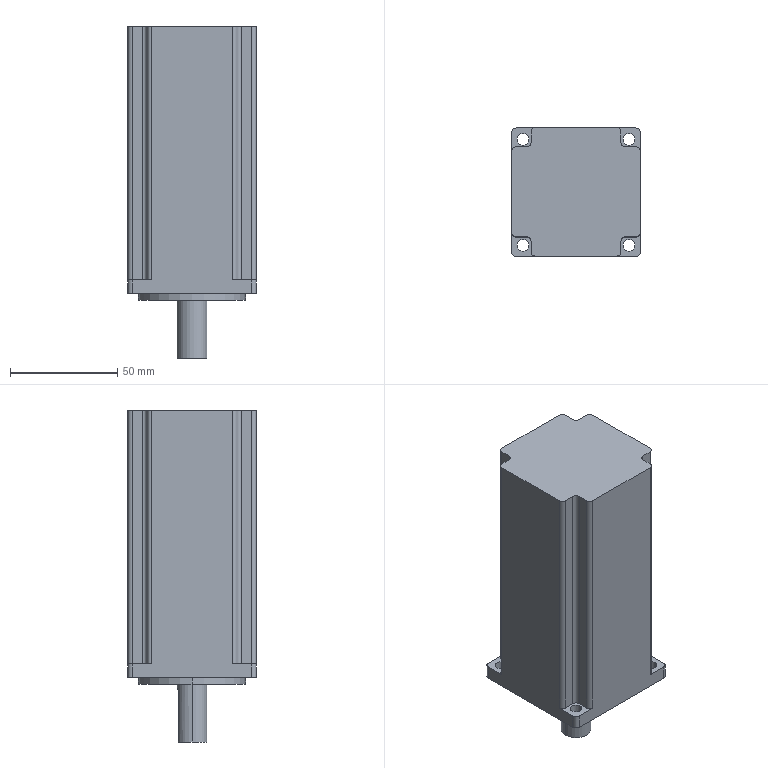Part | SolidWorks | features ICE 4, HoleWzd 2, MirrorPattern 2, Extrusion 1, Fillet 1 | 1 solid | 57 faces | box 60 x 60 x 155 mm | volume 420102 mm3 | cylinder 32 | plane 23 | cone 2 | commonest cylinder face diameters 4 x16 5.5 x8 4.2 x2 6 x2 14 x2 50 x2